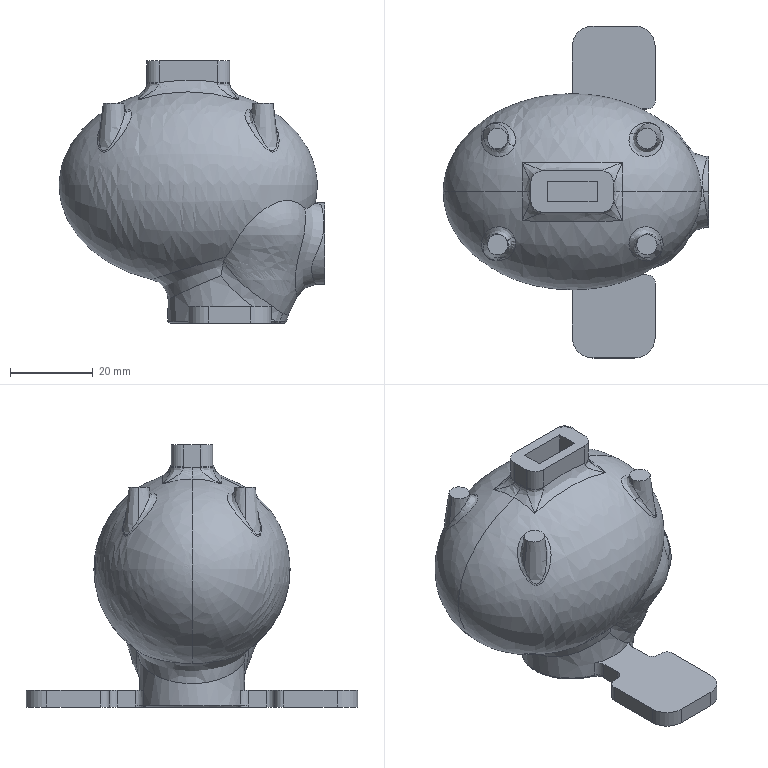Part | SolidWorks | features Fillet 4, ICE 2, BaseBody 1, BossThin 1, Cut 1, MirrorPattern 1 | 1 solid | 114 faces | box 63.97 x 80 x 63.184 mm | volume 89467 mm3 | spline 54 | plane 32 | cylinder 20 | cone 8 | commonest cylinder face diameters 4 x12 6 x4 10 x4